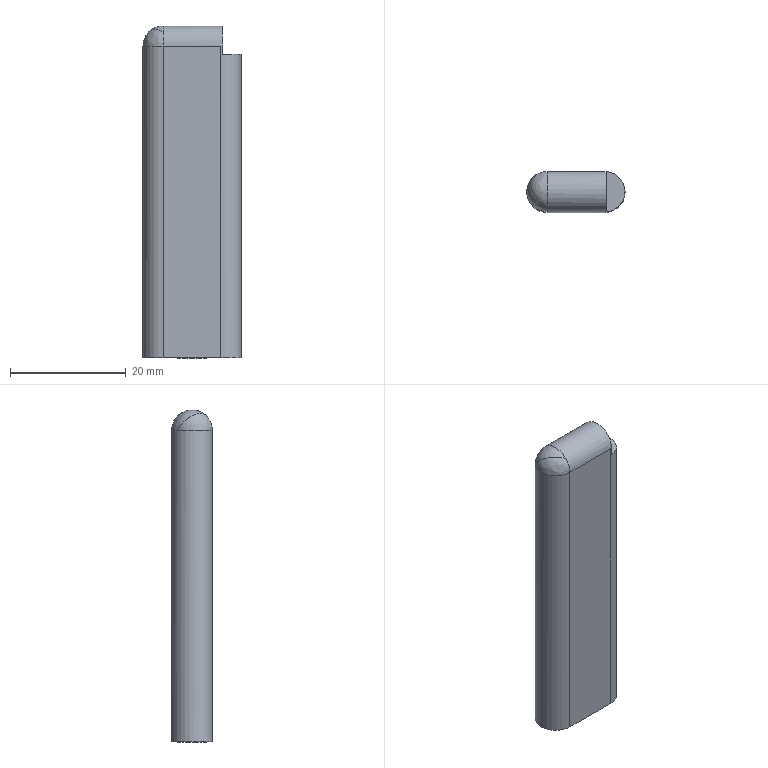Part | STEP file | LUOI GA TRON PHIA TREN | 1 solid | 17 faces | box 17 x 7 x 57.44 mm | volume 5792 mm3 | cylinder 6 | plane 5 | cone 4 | spline 2 | commonest cylinder face diameters 7 x4 4.134 x2